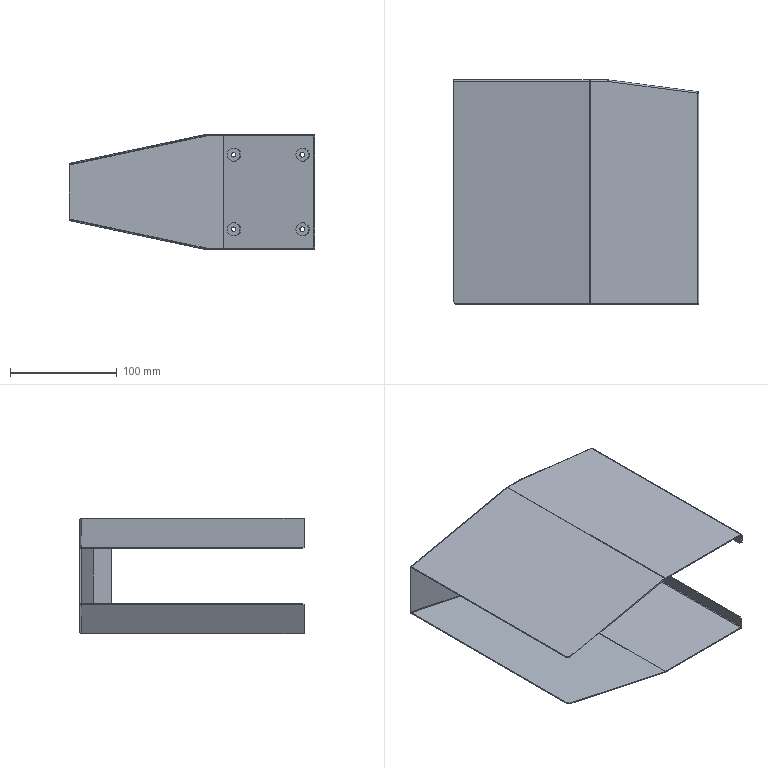Part | SolidWorks | features ICE 4, Chamfer 1, Extrusion 1, Fillet 1, HoleWzd 1, Shell 1 | 1 solid | 94 faces | box 230 x 210 x 108 mm | volume 125096 mm3 | cylinder 50 | plane 32 | sphere 12 | commonest cylinder face diameters 1 x12 3 x12 4.5 x8 8 x8 12 x8 20 x2